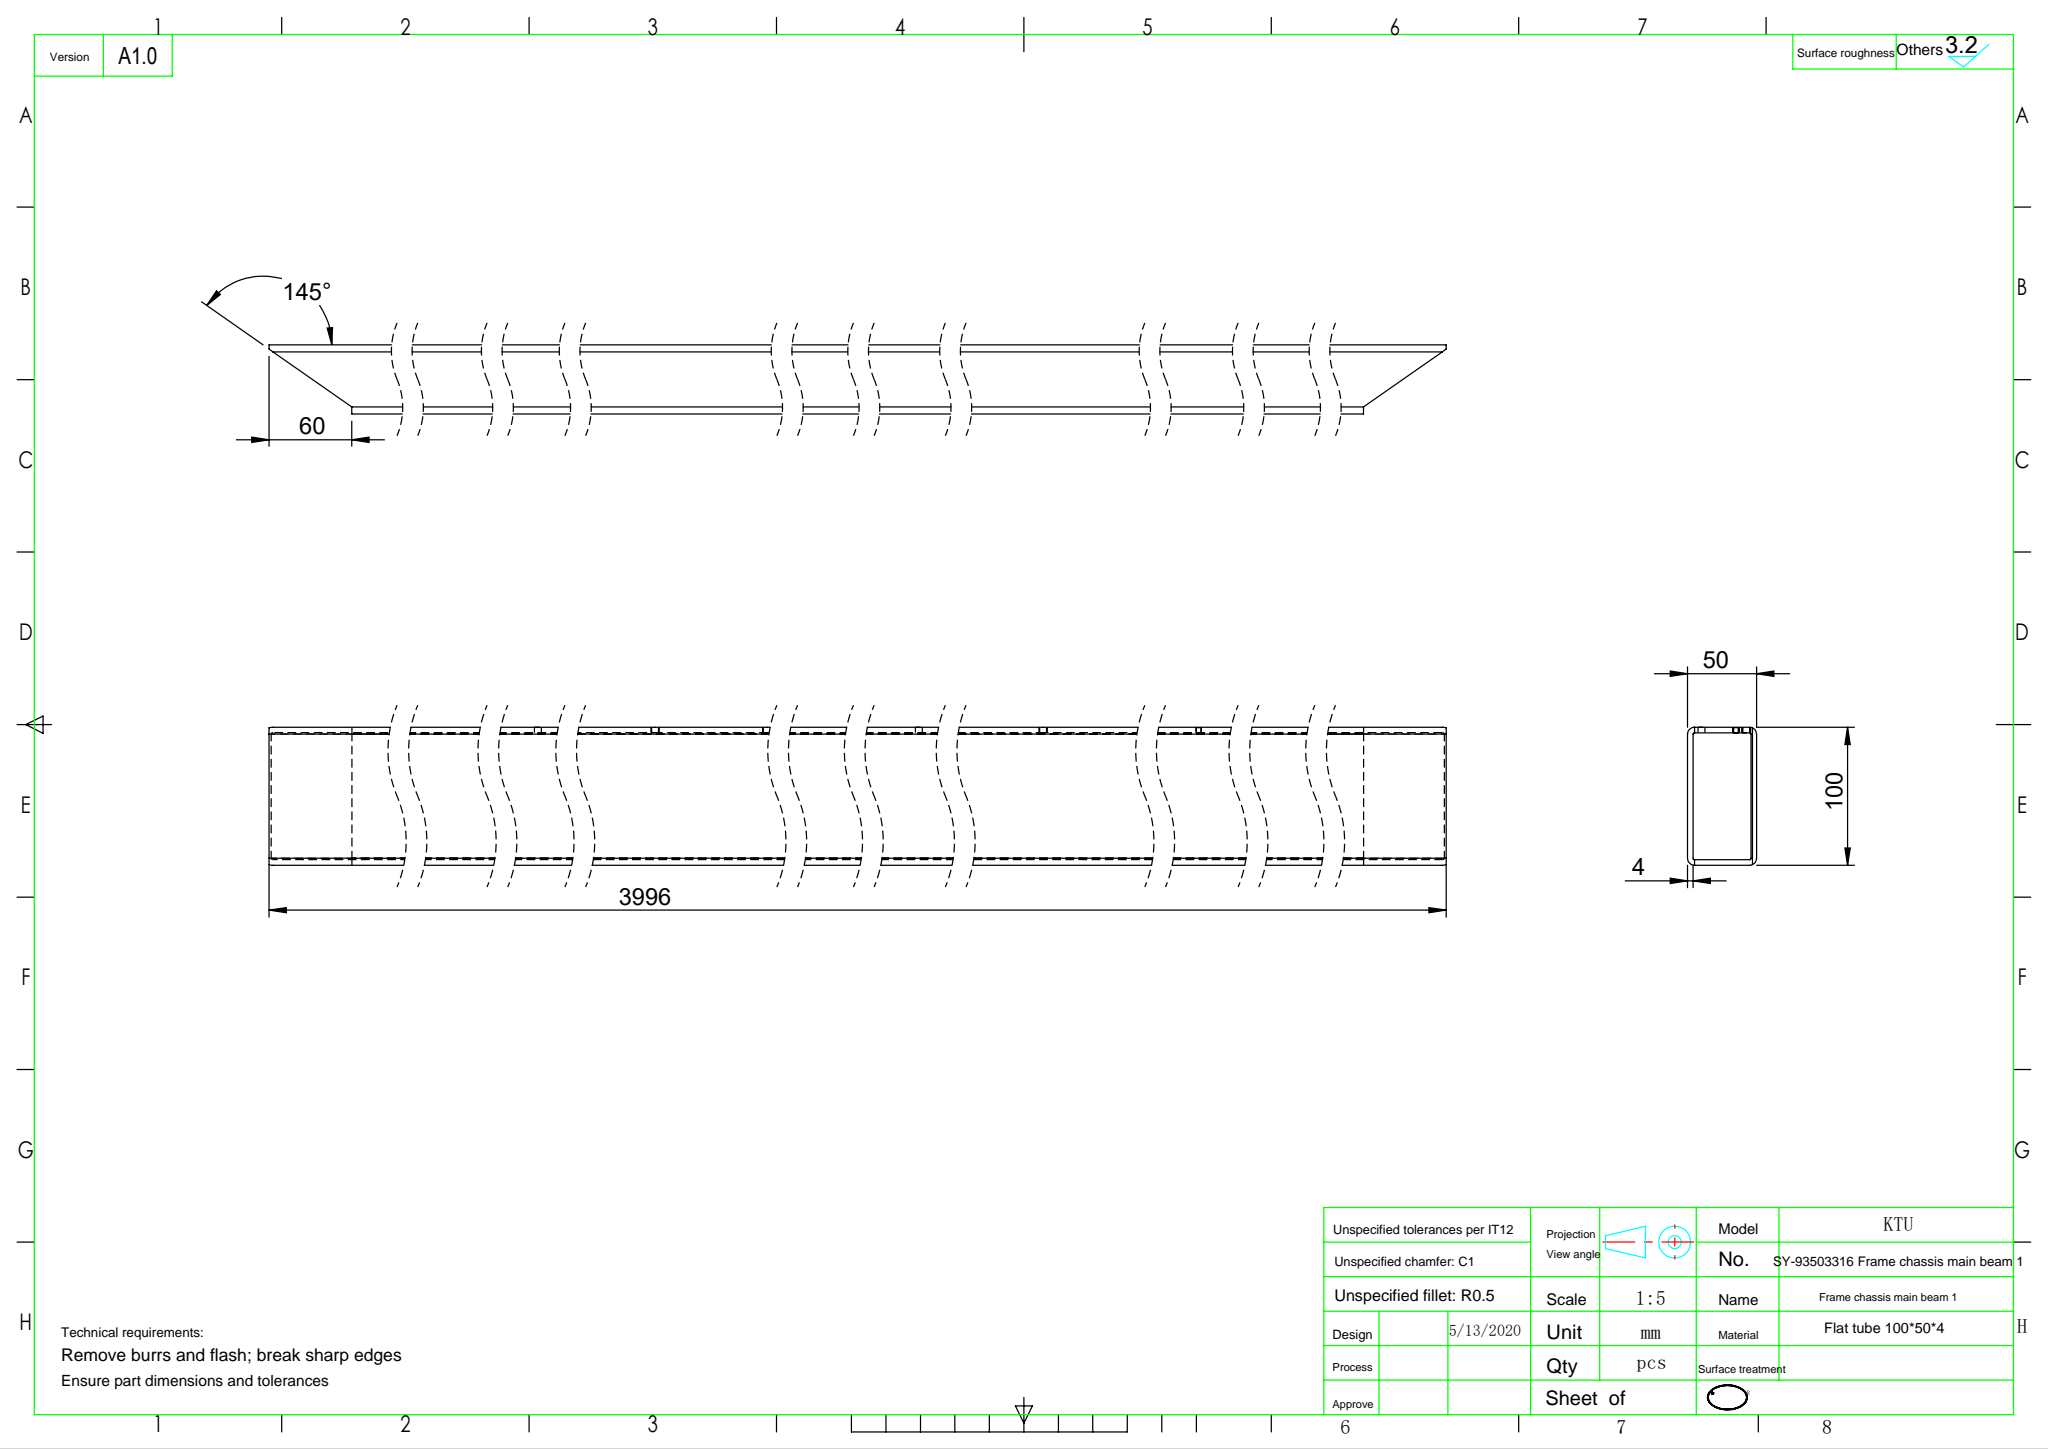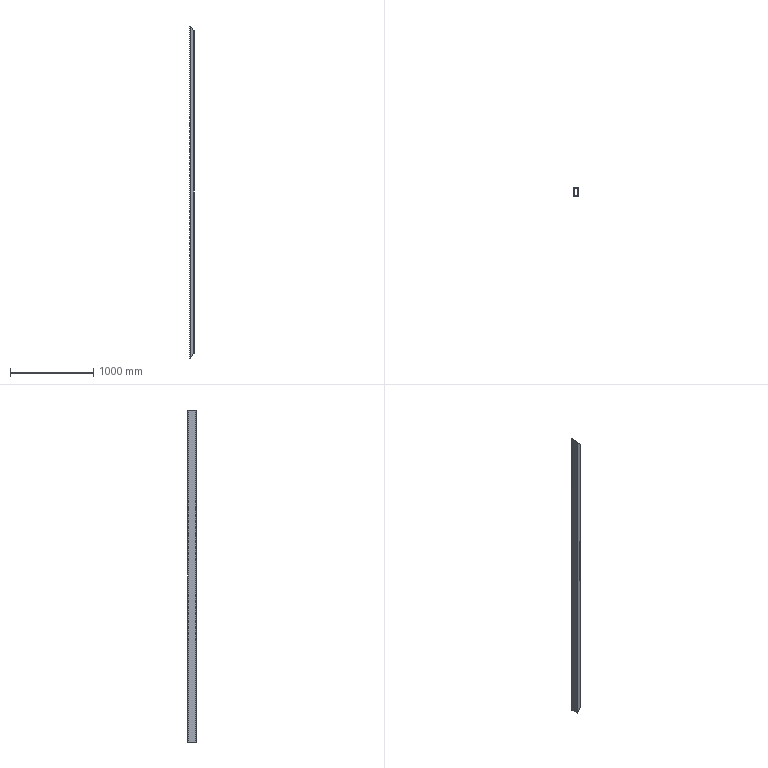Part | SolidWorks | features HoleWzd 4, ICE 3, CombineBodies 2, Cut 2, ExtruThin 1, LPattern 1 | 1 solid | 92 faces | box 50 x 100 x 3996 mm | volume 4387971 mm3 | cylinder 48 | cone 30 | plane 14 | commonest cylinder face diameters 3.3 x20 5 x20 2 x4 10 x4